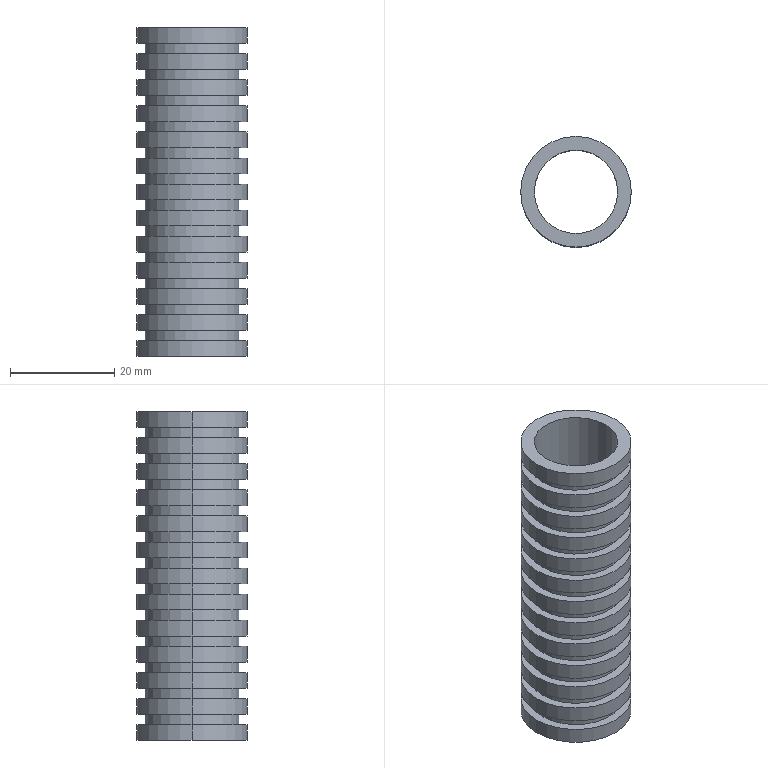Part | STEP file | P0177566_EZT_SCHUTZSCHLAUCH_MKR-16.5-PG-16 | 1 solid | 78 faces | box 21.2 x 21.2 x 63 mm | volume 7207 mm3 | cylinder 52 | plane 26 | commonest cylinder face diameters 21.2 x26 18 x24 16 x2